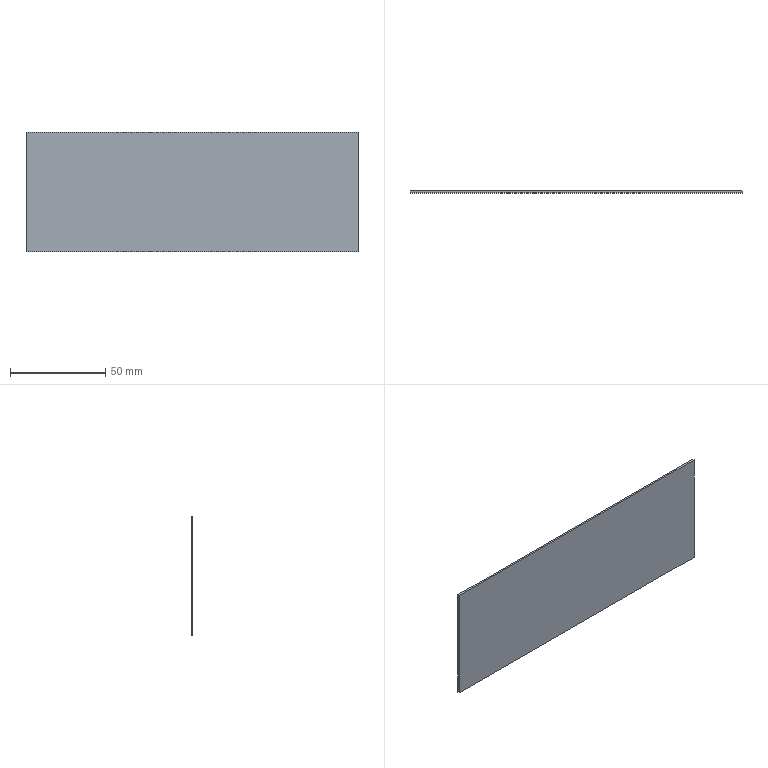Part | SolidWorks | features BaseBody 1 | 1 solid | 6 faces | box 174 x 1 x 62.5 mm | volume 10875 mm3 | plane 6
STEP:
#1=CARTESIAN_POINT('',(87.,-58.7,63.5));
#2=VERTEX_POINT('',#1);
#3=CARTESIAN_POINT('',(-87.,-58.7,63.5));
#4=VERTEX_POINT('',#3);
#5=CARTESIAN_POINT('',(0.,-58.7,63.5));
#6=DIRECTION('',(-1.,0.,0.));
#7=VECTOR('',#6,1000.);
#8=LINE('',#5,#7);
#9=EDGE_CURVE('',#2,#4,#8,.T.);
#10=ORIENTED_EDGE('',*,*,#9,.F.);
#11=CARTESIAN_POINT('',(87.,-58.7,1.));
#12=VERTEX_POINT('',#11);
#13=CARTESIAN_POINT('',(87.,-58.7,32.25));
#14=DIRECTION('',(0.,0.,1.));
#15=VECTOR('',#14,1000.);
#16=LINE('',#13,#15);
#17=EDGE_CURVE('',#12,#2,#16,.T.);
#18=ORIENTED_EDGE('',*,*,#17,.F.);
#19=CARTESIAN_POINT('',(-87.,-58.7,1.));
#20=VERTEX_POINT('',#19);
#21=CARTESIAN_POINT('',(0.,-58.7,1.));
#22=DIRECTION('',(1.,0.,0.));
#23=VECTOR('',#22,1000.);
#24=LINE('',#21,#23);
#25=EDGE_CURVE('',#20,#12,#24,.T.);
#26=ORIENTED_EDGE('',*,*,#25,.F.);
#27=CARTESIAN_POINT('',(-87.,-58.7,32.25));
#28=DIRECTION('',(0.,0.,-1.));
#29=VECTOR('',#28,1000.);
#30=LINE('',#27,#29);
#31=EDGE_CURVE('',#4,#20,#30,.T.);
#32=ORIENTED_EDGE('',*,*,#31,.F.);
#33=EDGE_LOOP('',(#10,#18,#26,#32));
#34=FACE_OUTER_BOUND('',#33,.T.);
#35=CARTESIAN_POINT('',(-90.48,-58.7,-0.25));
#36=DIRECTION('',(0.,-1.,0.));
#37=DIRECTION('',(1.,0.,0.));
#38=AXIS2_PLACEMENT_3D('',#35,#36,#37);
#39=PLANE('',#38);
#40=ADVANCED_FACE('',(#34),#39,.F.);
#41=CARTESIAN_POINT('',(-87.,-59.7,1.));
#42=VERTEX_POINT('',#41);
#43=CARTESIAN_POINT('',(-87.,-59.7,63.5));
#44=VERTEX_POINT('',#43);
#45=CARTESIAN_POINT('',(-87.,-59.7,32.25));
#46=DIRECTION('',(0.,0.,1.));
#47=VECTOR('',#46,1000.);
#48=LINE('',#45,#47);
#49=EDGE_CURVE('',#42,#44,#48,.T.);
#50=ORIENTED_EDGE('',*,*,#49,.T.);
#51=CARTESIAN_POINT('',(-87.,-59.2,63.5));
#52=DIRECTION('',(0.,1.,0.));
#53=VECTOR('',#52,1000.);
#54=LINE('',#51,#53);
#55=EDGE_CURVE('',#44,#4,#54,.T.);
#56=ORIENTED_EDGE('',*,*,#55,.T.);
#57=ORIENTED_EDGE('',*,*,#31,.T.);
#58=CARTESIAN_POINT('',(-87.,-59.2,1.));
#59=DIRECTION('',(0.,-1.,0.));
#60=VECTOR('',#59,1000.);
#61=LINE('',#58,#60);
#62=EDGE_CURVE('',#20,#42,#61,.T.);
#63=ORIENTED_EDGE('',*,*,#62,.T.);
#64=EDGE_LOOP('',(#50,#56,#57,#63));
#65=FACE_OUTER_BOUND('',#64,.T.);
#66=CARTESIAN_POINT('',(-87.,-58.472,64.75));
#67=DIRECTION('',(-1.,0.,0.));
#68=DIRECTION('',(0.,0.,-1.));
#69=AXIS2_PLACEMENT_3D('',#66,#67,#68);
#70=PLANE('',#69);
#71=ADVANCED_FACE('',(#65),#70,.T.);
#72=CARTESIAN_POINT('',(87.,-59.7,63.5));
#73=VERTEX_POINT('',#72);
#74=CARTESIAN_POINT('',(0.,-59.7,63.5));
#75=DIRECTION('',(1.,0.,0.));
#76=VECTOR('',#75,1000.);
#77=LINE('',#74,#76);
#78=EDGE_CURVE('',#44,#73,#77,.T.);
#79=ORIENTED_EDGE('',*,*,#78,.T.);
#80=CARTESIAN_POINT('',(87.,-59.2,63.5));
#81=DIRECTION('',(0.,1.,0.));
#82=VECTOR('',#81,1000.);
#83=LINE('',#80,#82);
#84=EDGE_CURVE('',#73,#2,#83,.T.);
#85=ORIENTED_EDGE('',*,*,#84,.T.);
#86=ORIENTED_EDGE('',*,*,#9,.T.);
#87=ORIENTED_EDGE('',*,*,#55,.F.);
#88=EDGE_LOOP('',(#79,#85,#86,#87));
#89=FACE_OUTER_BOUND('',#88,.T.);
#90=CARTESIAN_POINT('',(90.48,-58.472,63.5));
#91=DIRECTION('',(0.,0.,1.));
#92=DIRECTION('',(-1.,0.,0.));
#93=AXIS2_PLACEMENT_3D('',#90,#91,#92);
#94=PLANE('',#93);
#95=ADVANCED_FACE('',(#89),#94,.T.);
#96=CARTESIAN_POINT('',(87.,-59.7,1.));
#97=VERTEX_POINT('',#96);
#98=CARTESIAN_POINT('',(87.,-59.7,32.25));
#99=DIRECTION('',(0.,0.,-1.));
#100=VECTOR('',#99,1000.);
#101=LINE('',#98,#100);
#102=EDGE_CURVE('',#73,#97,#101,.T.);
#103=ORIENTED_EDGE('',*,*,#102,.T.);
#104=CARTESIAN_POINT('',(87.,-59.2,1.));
#105=DIRECTION('',(0.,1.,0.));
#106=VECTOR('',#105,1000.);
#107=LINE('',#104,#106);
#108=EDGE_CURVE('',#97,#12,#107,.T.);
#109=ORIENTED_EDGE('',*,*,#108,.T.);
#110=ORIENTED_EDGE('',*,*,#17,.T.);
#111=ORIENTED_EDGE('',*,*,#84,.F.);
#112=EDGE_LOOP('',(#103,#109,#110,#111));
#113=FACE_OUTER_BOUND('',#112,.T.);
#114=CARTESIAN_POINT('',(87.,-58.472,-0.25));
#115=DIRECTION('',(1.,0.,0.));
#116=DIRECTION('',(0.,0.,1.));
#117=AXIS2_PLACEMENT_3D('',#114,#115,#116);
#118=PLANE('',#117);
#119=ADVANCED_FACE('',(#113),#118,.T.);
#120=CARTESIAN_POINT('',(0.,-59.7,1.));
#121=DIRECTION('',(-1.,0.,0.));
#122=VECTOR('',#121,1000.);
#123=LINE('',#120,#122);
#124=EDGE_CURVE('',#97,#42,#123,.T.);
#125=ORIENTED_EDGE('',*,*,#124,.T.);
#126=ORIENTED_EDGE('',*,*,#62,.F.);
#127=ORIENTED_EDGE('',*,*,#25,.T.);
#128=ORIENTED_EDGE('',*,*,#108,.F.);
#129=EDGE_LOOP('',(#125,#126,#127,#128));
#130=FACE_OUTER_BOUND('',#129,.T.);
#131=CARTESIAN_POINT('',(-90.48,-58.472,1.));
#132=DIRECTION('',(0.,0.,-1.));
#133=DIRECTION('',(1.,0.,0.));
#134=AXIS2_PLACEMENT_3D('',#131,#132,#133);
#135=PLANE('',#134);
#136=ADVANCED_FACE('',(#130),#135,.T.);
#137=ORIENTED_EDGE('',*,*,#78,.F.);
#138=ORIENTED_EDGE('',*,*,#49,.F.);
#139=ORIENTED_EDGE('',*,*,#124,.F.);
#140=ORIENTED_EDGE('',*,*,#102,.F.);
#141=EDGE_LOOP('',(#137,#138,#139,#140));
#142=FACE_OUTER_BOUND('',#141,.T.);
#143=CARTESIAN_POINT('',(-90.48,-59.7,-0.25));
#144=DIRECTION('',(0.,-1.,0.));
#145=DIRECTION('',(1.,0.,0.));
#146=AXIS2_PLACEMENT_3D('',#143,#144,#145);
#147=PLANE('',#146);
#148=ADVANCED_FACE('',(#142),#147,.T.);
#149=CLOSED_SHELL('',(#40,#71,#95,#119,#136,#148));
#150=MANIFOLD_SOLID_BREP('',#149);
#151=CARTESIAN_POINT('',(0.,0.,0.));
#152=DIRECTION('',(0.,0.,1.));
#153=DIRECTION('',(1.,0.,0.));
#154=AXIS2_PLACEMENT_3D('',#151,#152,#153);
#155=(LENGTH_UNIT()NAMED_UNIT(*)SI_UNIT(.MILLI.,.METRE.));
#156=UNCERTAINTY_MEASURE_WITH_UNIT(LENGTH_MEASURE(0.00001),#155,'','');
#157=(NAMED_UNIT(*)PLANE_ANGLE_UNIT()SI_UNIT($,.RADIAN.));
#158=(NAMED_UNIT(*)SI_UNIT($,.STERADIAN.)SOLID_ANGLE_UNIT());
#159=(GEOMETRIC_REPRESENTATION_CONTEXT(3)GLOBAL_UNCERTAINTY_ASSIGNED_CONTEXT((#156))GLOBAL_UNIT_ASSIGNED_CONTEXT((#155,#157,#158))REPRESENTATION_CONTEXT('',''));
#160=ADVANCED_BREP_SHAPE_REPRESENTATION('',(#150,#154),#159);